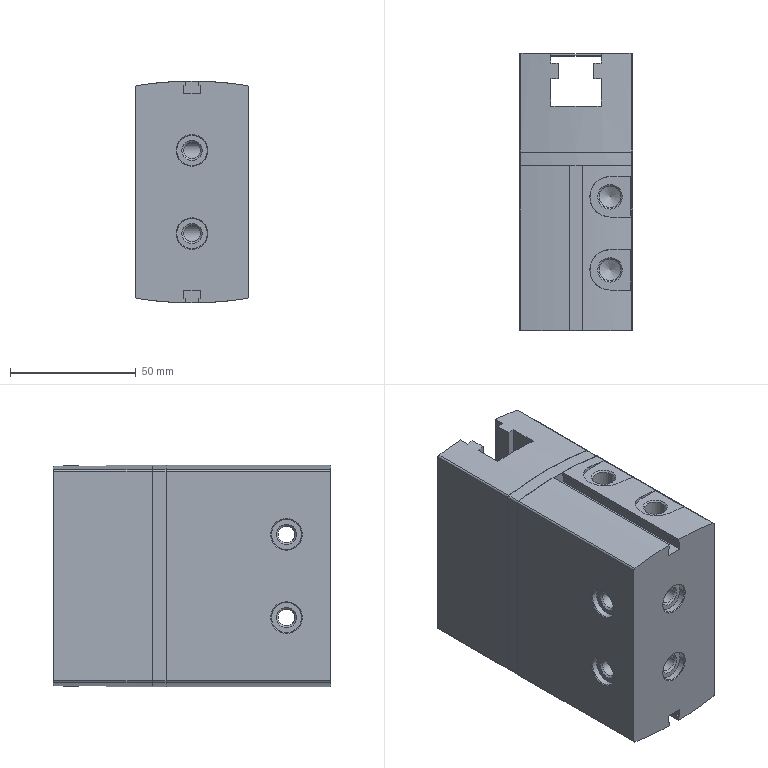Part | STEP file | 1254052_DHPS_35_A_2_14a---(CORPO) | 1 solid | 125 faces | box 45 x 110 x 88 mm | volume 385096 mm3 | plane 71 | cylinder 38 | cone 16 | commonest cylinder face diameters 1.4 x12 12 x6 270 x6 2.2 x4 6.647 x4 8.566 x2